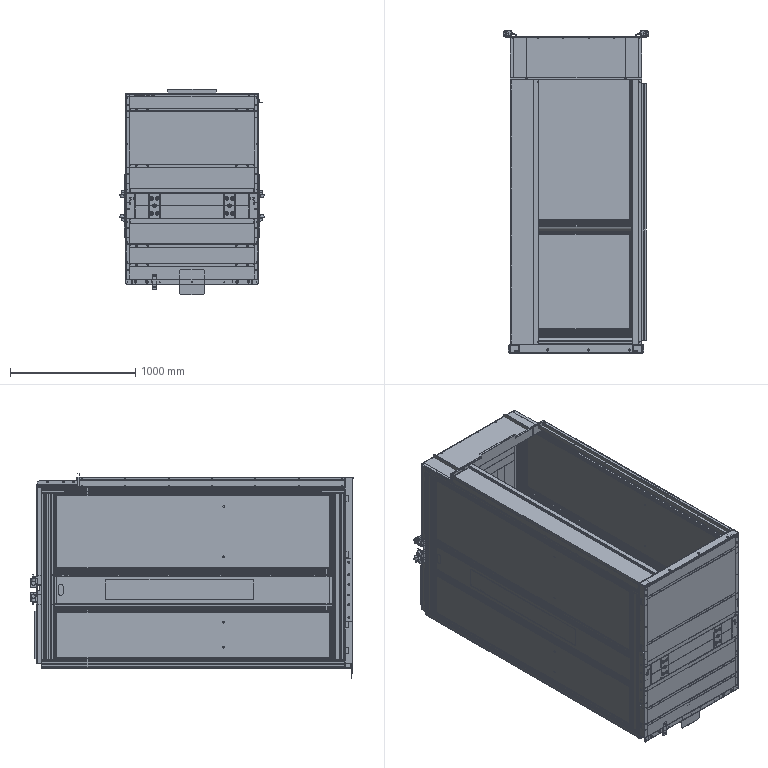Part | SolidWorks | 334 solids | 11520 faces | volume 247371148 mm3 | plane 7310 | cylinder 3958 | cone 252 | commonest cylinder face diameters 6 x383 10 x349 11 x291 0.4 x281 1.1 x240 8.5 x220